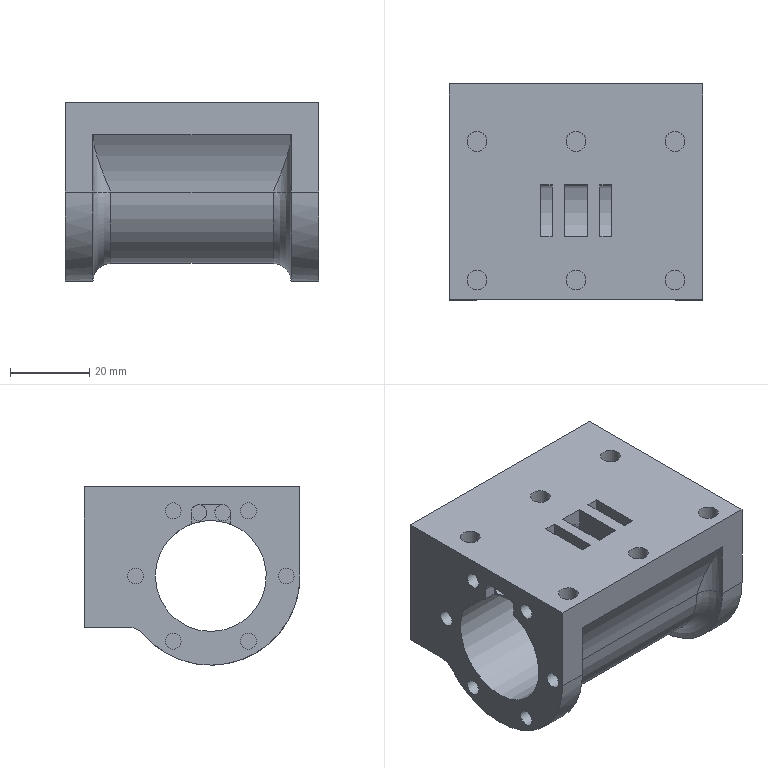Part | STEP file | 1-06.1 | 1 solid | 92 faces | box 64 x 54.5 x 45 mm | volume 79802 mm3 | plane 51 | cylinder 39 | spline 2 | commonest cylinder face diameters 4 x16 5 x11 9 x4 45 x2 6 x1 10 x1